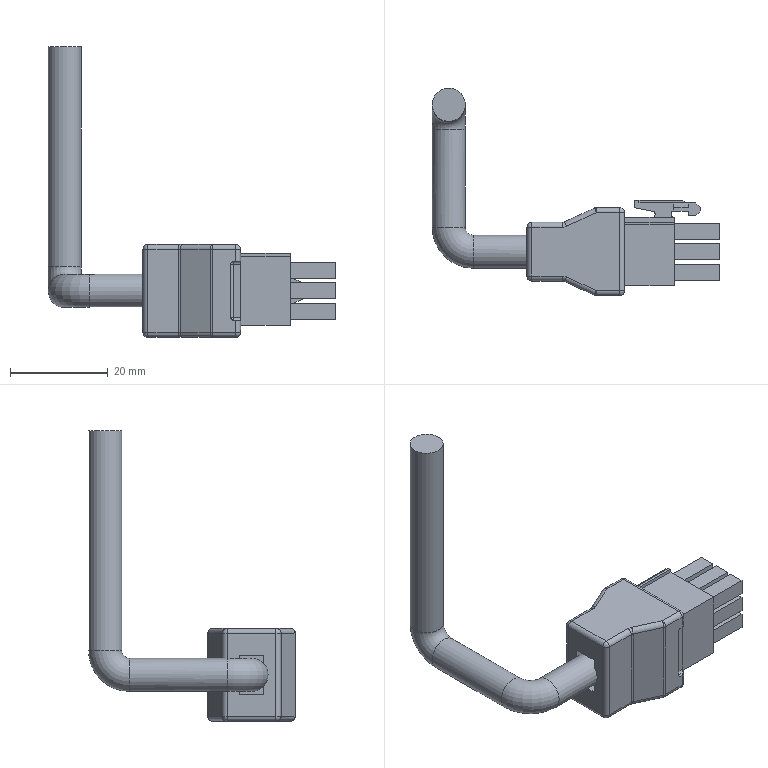Part | STEP file | 1 solid | 171 faces | box 58.9 x 42.4 x 59.5 mm | volume 11878 mm3 | plane 107 | cylinder 41 | sphere 16 | torus 6 | spline 1 | commonest cylinder face diameters 2 x26 1 x10 6.8 x3 1.3 x2